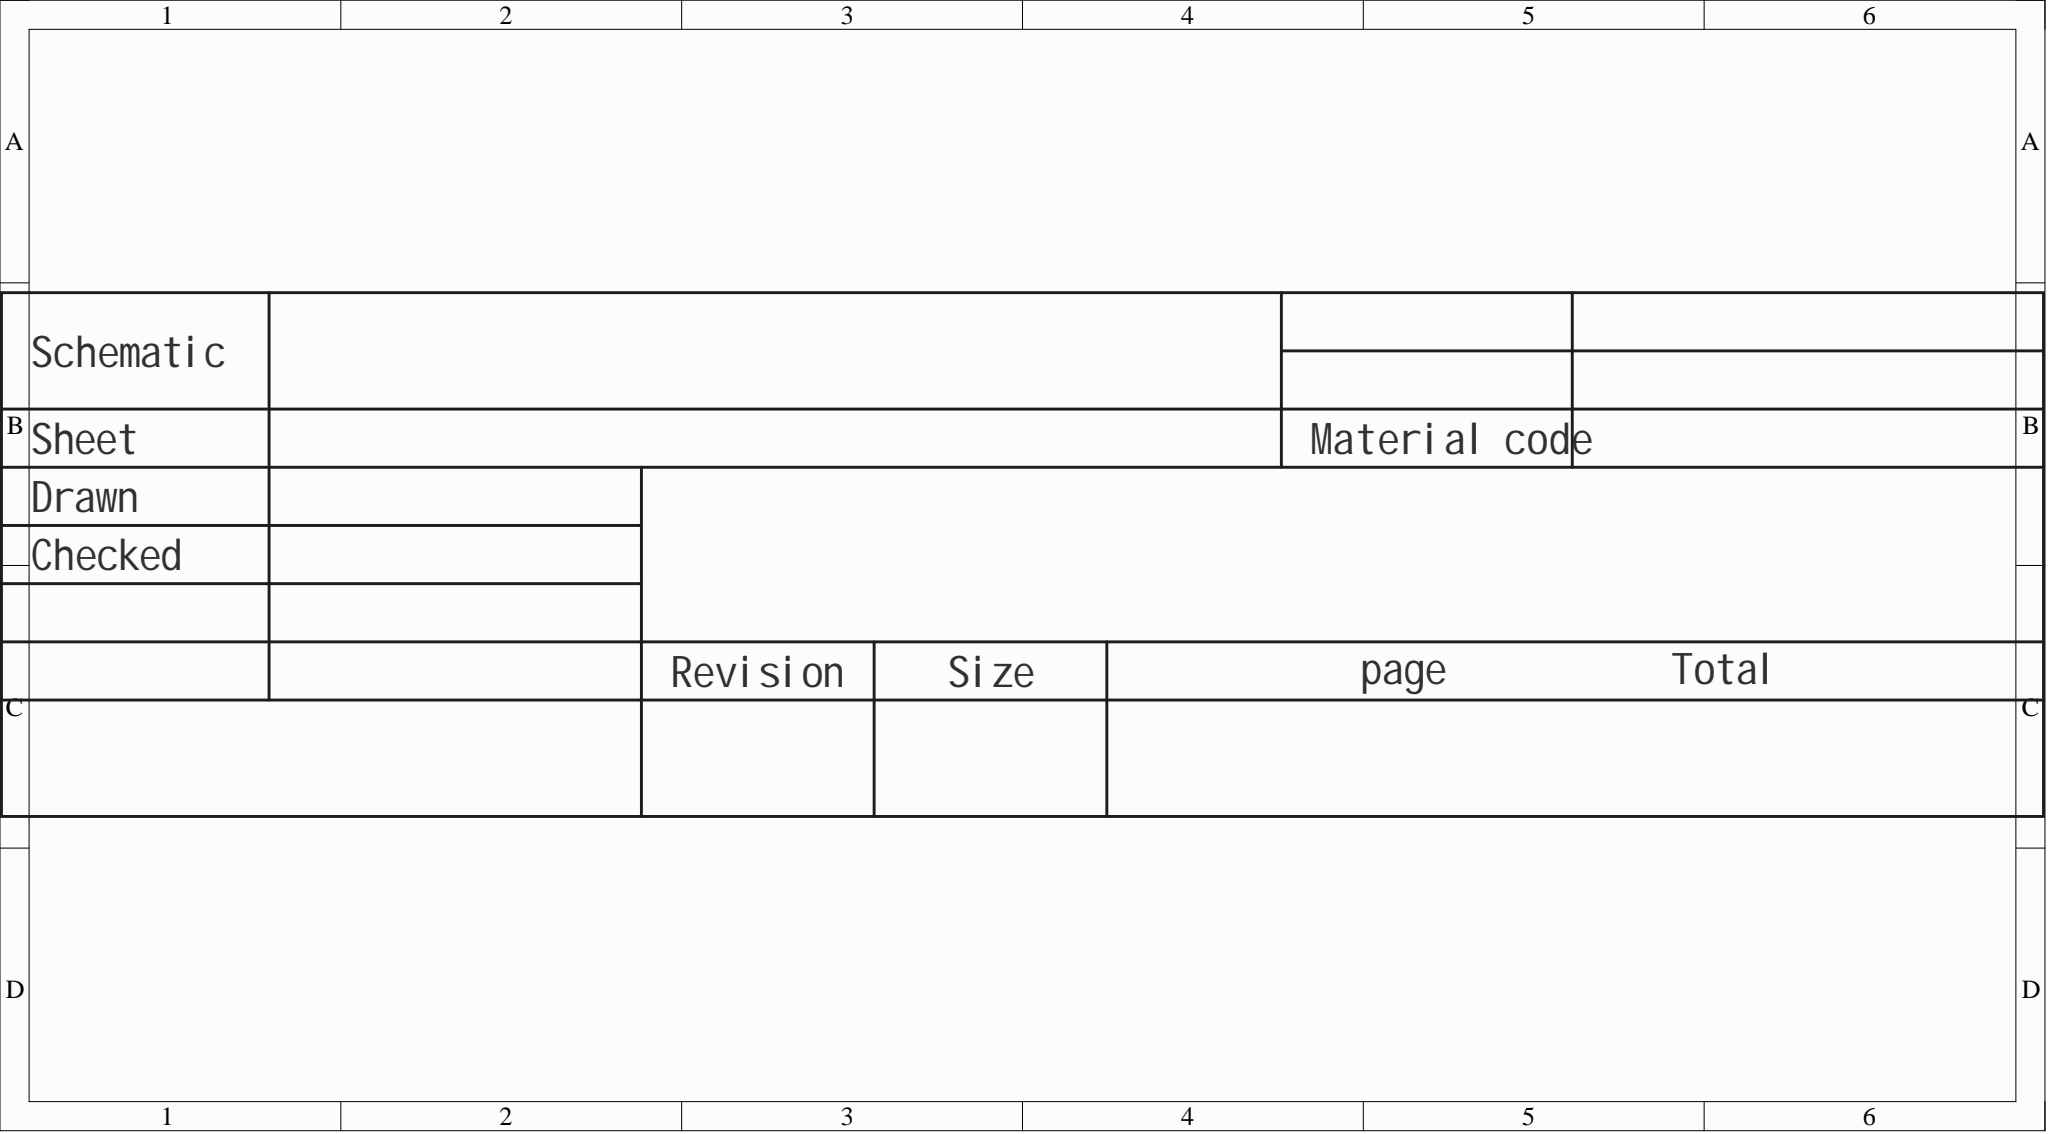Circuit board | Altium Designer | 29 parts | 34 nets
Bill of materials:
Comment,Description,Designator,Footprint,LibRef,Quantity
"buzzer-12X9","","BUZZER1","BUZ-TH_BD12.0-P7.60-D0.6-FD","buzzer-12X9","1"
"10uf","","C1","C0805","CAP_0805","1"
"30pf","","C2, C3","C0805","CAP_0805","2"
"","","H1","HDR-TH_9P-P2.54-V-F-1","HDR-F_2.54_1x9P","1"
"","","H2, H3, H6","HDR-TH_3P-P2.54-V-F","HDR-F_2.54_1x3P","3"
"","","H4","HDR-TH_4P-P2.54-V-F","HDR-F_2.54_1x4P","1"
"","","H5","HDR-TH_2P-P2.54-V-M-1","HDR-M_2.54_1x2P","1"
"LMB162ADC","16x2 character LCD module","LCD1","LCD1602","LMB162ADC","1"
"","","LEDG1, LEDG2, LEDR1","LED_0805","LED_0805-R","3"
"2N3906S-RTK/PS","","Q1","SOT-23-3_L2.9-W1.3-P1.90-LS2.4-TR","2N3906S-RTK/PS","1"
"10K","","R1, R2","R0805","Res_0805","2"
"1K","","R3","R0805","Res_0805","1"
"220","","R4, R5, R7","R0805","Res_0805","3"
"2.2K","","R6","R0805","Res_0805","1"
"Tact switch 3*6*2.5","","SW1, SW2, SW3, SW4","SW-SMD_L6.0-W3.6-LS8.0","轻触按键3*6*2.5","4"
"STC89C516RD+40I-PDIP40","CPU core: 51 series; program memory: 61KB; total RAM: 1.25KB; GPIO count: 35; operating voltage: 3.5V~5.5V; max CPU frequency: -; program memory type: FLASH;","U1","DIP-40_L52.3-W13.9-P2.54-LS15.2-BL","STC89C516RD+40I-PDIP40","1"
"11.059MHz","Frequency: 12MHz; room-temp tolerance: ±30ppm; external load capacitance: -; stability (full temp): ±50ppm;","U2","HC-49US_L11.0-W4.6-P4.88","ECS-120-S-4","1"
"Ai-Thinker ESP-01S ESP8266","","U3","WIFIM-TH_8P-L24.7-W14.4-P2.54","Ai-Thinker ESP-01S ESP8266","1"
Netlist (Protel format):
[
BUZZER1
BUZ-TH_BD12.0-P7.60-D0.6-FD
buzzer-12X9



]
[
C1
C0805
10uf



]
[
C2
C0805
30pf



]
[
C3
C0805
30pf



]
[
H1
HDR-TH_9P-P2.54-V-F-1




]
[
H2
HDR-TH_3P-P2.54-V-F




]
[
H3
HDR-TH_3P-P2.54-V-F




]
[
H4
HDR-TH_4P-P2.54-V-F




]
[
H5
HDR-TH_2P-P2.54-V-M-1




]
[
H6
HDR-TH_3P-P2.54-V-F




]
[
LCD1
LCD1602
LMB162ADC



]
[
LEDG1
LED_0805




]
[
LEDG2
LED_0805




]
[
LEDR1
LED_0805




]
[
Q1
SOT-23-3_L2.9-W1.3-P1.90-LS2.4-TR
2N3906S-RTK/PS



]
[
R1
R0805
10K



]
[
R2
R0805
10K



]
[
R3
R0805
1K



]
[
R4
R0805
220



]
[
R5
R0805
220



]
[
R6
R0805
2.2K



]
[
R7
R0805
220



]
[
SW1
SW-SMD_L6.0-W3.6-LS8.0
Tact switch 3*6*2.5



]
[
SW2
SW-SMD_L6.0-W3.6-LS8.0
Tact switch 3*6*2.5



]
[
SW3
SW-SMD_L6.0-W3.6-LS8.0
Tact switch 3*6*2.5



]
[
SW4
SW-SMD_L6.0-W3.6-LS8.0
Tact switch 3*6*2.5



]
[
U1
DIP-40_L52.3-W13.9-P2.54-LS15.2-BL
STC89C516RD+40I-PDIP40



]
[
U2
HC-49US_L11.0-W4.6-P4.88
11.0592MHz



]
[
U3
WIFIM-TH_8P-L24.7-W14.4-P2.54
Ai-Thinker ESP-01S ESP8266



]
(
VCC
BUZZER1-2
C1-2
H1-1
H2-1
H3-1
H4-3
H5-2
H6-1
LCD1-2
LCD1-15
R2-2
R4-2
R5-2
R7-2
SW1-2
U1-40
U3-8
)
(
TX0
U1-11
U3-4
)
(
RX0
U1-10
U3-5
)
(
RS
LCD1-4
U1-24
)
(
NetSW4_1
SW4-1
U1-17
)
(
NetSW3_1
SW3-1
U1-28
)
(
NetSW2_1
SW2-1
U1-27
)
(
NetR6_1
R6-1
U1-26
)
(
NetQ1_2
Q1-2
R6-2
)
(
NetLEDR1_2
LEDR1-2
R4-1
)
(
NetLEDR1_1
LEDR1-1
U1-23
)
(
NetLEDG2_2
LEDG2-2
R7-1
)
(
NetLEDG1_2
LEDG1-2
R5-1
)
(
NetLEDG1_1
LEDG1-1
U1-21
)
(
NetLCD1_3
LCD1-3
R2-1
R3-2
)
(
NetH6_2
H6-2
U1-1
)
(
NetH4_2
H4-2
U1-30
)
(
NetH4_1
H4-1
U1-31
)
(
NetH3_2
H3-2
U1-3
)
(
NetH2_2
H2-2
U1-13
)
(
NetH1_9
H1-9
LCD1-14
U1-32
)
(
NetH1_8
H1-8
LCD1-13
U1-33
)
(
NetH1_7
H1-7
LCD1-12
U1-34
)
(
NetH1_6
H1-6
LCD1-11
U1-35
)
(
NetH1_5
H1-5
LCD1-10
U1-36
)
(
NetH1_4
H1-4
LCD1-9
U1-37
)
(
NetH1_3
H1-3
LCD1-8
U1-38
)
(
NetH1_2
H1-2
LCD1-7
U1-39
)
(
NetC3_2
C3-2
U1-19
U2-2
)
(
NetC2_2
C2-2
U1-18
U2-1
)
(
NetC1_1
C1-1
R1-1
SW1-1
U1-9
)
(
NetBUZZER1_1
BUZZER1-1
Q1-1
)
(
GND
C2-1
C3-1
H2-3
H3-3
H4-4
H5-1
H6-3
LCD1-1
LCD1-5
LCD1-16
LEDG2-1
Q1-3
R1-2
R3-1
SW2-2
SW3-2
SW4-2
U1-20
U3-1
)
(
EN
LCD1-6
U1-25
)